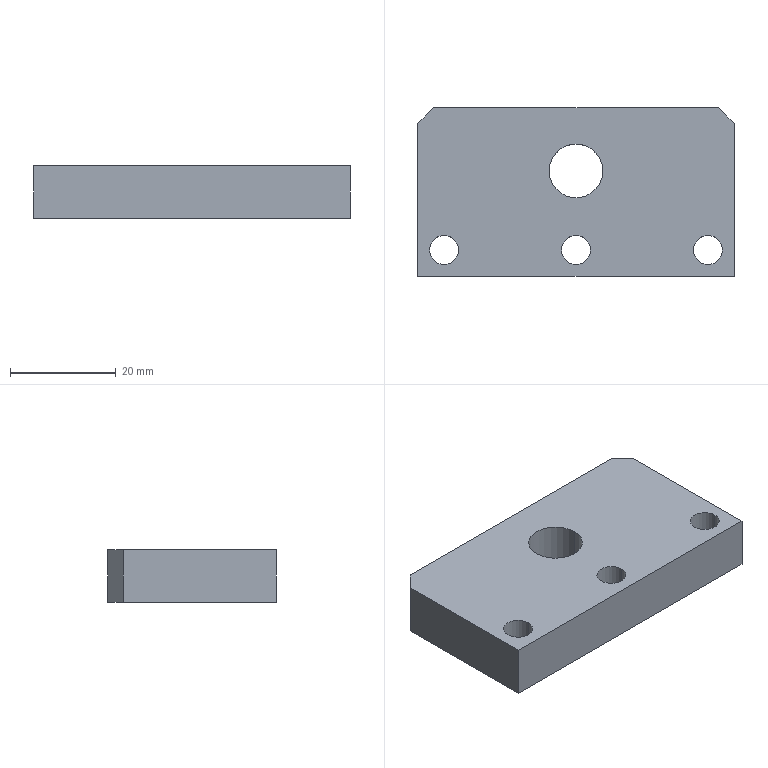Part | STEP file | MT-COMBO-119-S030 | 1 solid | 16 faces | box 60 x 32 x 10 mm | volume 17580 mm3 | cylinder 8 | plane 8 | commonest cylinder face diameters 5.5 x6 10.2 x2
STEP:
#1=CARTESIAN_POINT('',(-22.25,-11.,5.));
#2=VERTEX_POINT('',#1);
#3=CARTESIAN_POINT('',(-27.75,-11.,5.));
#4=VERTEX_POINT('',#3);
#5=CARTESIAN_POINT('',(-25.,-11.,5.));
#6=DIRECTION('',(0.,0.,1.));
#7=DIRECTION('',(1.,0.,0.));
#8=AXIS2_PLACEMENT_3D('',#5,#6,#7);
#9=CIRCLE('',#8,2.75);
#10=EDGE_CURVE('',#2,#4,#9,.T.);
#11=ORIENTED_EDGE('',*,*,#10,.T.);
#12=CARTESIAN_POINT('',(-27.75,-11.,-5.));
#13=VERTEX_POINT('',#12);
#14=CARTESIAN_POINT('',(-27.75,-11.,-5.));
#15=DIRECTION('',(0.,0.,-1.));
#16=VECTOR('',#15,1000.);
#17=LINE('',#14,#16);
#18=EDGE_CURVE('',#4,#13,#17,.T.);
#19=ORIENTED_EDGE('',*,*,#18,.T.);
#20=CARTESIAN_POINT('',(-22.25,-11.,-5.));
#21=VERTEX_POINT('',#20);
#22=CARTESIAN_POINT('',(-25.,-11.,-5.));
#23=DIRECTION('',(0.,0.,1.));
#24=DIRECTION('',(1.,0.,0.));
#25=AXIS2_PLACEMENT_3D('',#22,#23,#24);
#26=CIRCLE('',#25,2.75);
#27=EDGE_CURVE('',#21,#13,#26,.T.);
#28=ORIENTED_EDGE('',*,*,#27,.F.);
#29=CARTESIAN_POINT('',(-22.25,-11.,-5.));
#30=DIRECTION('',(0.,0.,-1.));
#31=VECTOR('',#30,1000.);
#32=LINE('',#29,#31);
#33=EDGE_CURVE('',#2,#21,#32,.T.);
#34=ORIENTED_EDGE('',*,*,#33,.F.);
#35=EDGE_LOOP('',(#11,#19,#28,#34));
#36=FACE_OUTER_BOUND('',#35,.T.);
#37=CARTESIAN_POINT('',(-25.,-11.,-5.));
#38=DIRECTION('',(0.,0.,-1.));
#39=DIRECTION('',(1.,0.,0.));
#40=AXIS2_PLACEMENT_3D('',#37,#38,#39);
#41=CYLINDRICAL_SURFACE('',#40,2.75);
#42=ADVANCED_FACE('',(#36),#41,.F.);
#43=CARTESIAN_POINT('',(27.75,-11.,5.));
#44=VERTEX_POINT('',#43);
#45=CARTESIAN_POINT('',(22.25,-11.,5.));
#46=VERTEX_POINT('',#45);
#47=CARTESIAN_POINT('',(25.,-11.,5.));
#48=DIRECTION('',(0.,0.,1.));
#49=DIRECTION('',(1.,0.,0.));
#50=AXIS2_PLACEMENT_3D('',#47,#48,#49);
#51=CIRCLE('',#50,2.75);
#52=EDGE_CURVE('',#44,#46,#51,.T.);
#53=ORIENTED_EDGE('',*,*,#52,.T.);
#54=CARTESIAN_POINT('',(22.25,-11.,-5.));
#55=VERTEX_POINT('',#54);
#56=CARTESIAN_POINT('',(22.25,-11.,-5.));
#57=DIRECTION('',(0.,0.,-1.));
#58=VECTOR('',#57,1000.);
#59=LINE('',#56,#58);
#60=EDGE_CURVE('',#46,#55,#59,.T.);
#61=ORIENTED_EDGE('',*,*,#60,.T.);
#62=CARTESIAN_POINT('',(27.75,-11.,-5.));
#63=VERTEX_POINT('',#62);
#64=CARTESIAN_POINT('',(25.,-11.,-5.));
#65=DIRECTION('',(0.,0.,1.));
#66=DIRECTION('',(1.,0.,0.));
#67=AXIS2_PLACEMENT_3D('',#64,#65,#66);
#68=CIRCLE('',#67,2.75);
#69=EDGE_CURVE('',#63,#55,#68,.T.);
#70=ORIENTED_EDGE('',*,*,#69,.F.);
#71=CARTESIAN_POINT('',(27.75,-11.,-5.));
#72=DIRECTION('',(0.,0.,-1.));
#73=VECTOR('',#72,1000.);
#74=LINE('',#71,#73);
#75=EDGE_CURVE('',#44,#63,#74,.T.);
#76=ORIENTED_EDGE('',*,*,#75,.F.);
#77=EDGE_LOOP('',(#53,#61,#70,#76));
#78=FACE_OUTER_BOUND('',#77,.T.);
#79=CARTESIAN_POINT('',(25.,-11.,-5.));
#80=DIRECTION('',(0.,0.,-1.));
#81=DIRECTION('',(1.,0.,0.));
#82=AXIS2_PLACEMENT_3D('',#79,#80,#81);
#83=CYLINDRICAL_SURFACE('',#82,2.75);
#84=ADVANCED_FACE('',(#78),#83,.F.);
#85=CARTESIAN_POINT('',(2.75,-11.,5.));
#86=VERTEX_POINT('',#85);
#87=CARTESIAN_POINT('',(-2.75,-11.,5.));
#88=VERTEX_POINT('',#87);
#89=CARTESIAN_POINT('',(0.,-11.,5.));
#90=DIRECTION('',(0.,0.,1.));
#91=DIRECTION('',(1.,0.,0.));
#92=AXIS2_PLACEMENT_3D('',#89,#90,#91);
#93=CIRCLE('',#92,2.75);
#94=EDGE_CURVE('',#86,#88,#93,.T.);
#95=ORIENTED_EDGE('',*,*,#94,.T.);
#96=CARTESIAN_POINT('',(-2.75,-11.,-5.));
#97=VERTEX_POINT('',#96);
#98=CARTESIAN_POINT('',(-2.75,-11.,-5.));
#99=DIRECTION('',(0.,0.,-1.));
#100=VECTOR('',#99,1000.);
#101=LINE('',#98,#100);
#102=EDGE_CURVE('',#88,#97,#101,.T.);
#103=ORIENTED_EDGE('',*,*,#102,.T.);
#104=CARTESIAN_POINT('',(2.75,-11.,-5.));
#105=VERTEX_POINT('',#104);
#106=CARTESIAN_POINT('',(0.,-11.,-5.));
#107=DIRECTION('',(0.,0.,1.));
#108=DIRECTION('',(1.,0.,0.));
#109=AXIS2_PLACEMENT_3D('',#106,#107,#108);
#110=CIRCLE('',#109,2.75);
#111=EDGE_CURVE('',#105,#97,#110,.T.);
#112=ORIENTED_EDGE('',*,*,#111,.F.);
#113=CARTESIAN_POINT('',(2.75,-11.,-5.));
#114=DIRECTION('',(0.,0.,-1.));
#115=VECTOR('',#114,1000.);
#116=LINE('',#113,#115);
#117=EDGE_CURVE('',#86,#105,#116,.T.);
#118=ORIENTED_EDGE('',*,*,#117,.F.);
#119=EDGE_LOOP('',(#95,#103,#112,#118));
#120=FACE_OUTER_BOUND('',#119,.T.);
#121=CARTESIAN_POINT('',(0.,-11.,-5.));
#122=DIRECTION('',(0.,0.,-1.));
#123=DIRECTION('',(1.,0.,0.));
#124=AXIS2_PLACEMENT_3D('',#121,#122,#123);
#125=CYLINDRICAL_SURFACE('',#124,2.75);
#126=ADVANCED_FACE('',(#120),#125,.F.);
#127=CARTESIAN_POINT('',(5.1,4.,5.));
#128=VERTEX_POINT('',#127);
#129=CARTESIAN_POINT('',(-5.1,4.,5.));
#130=VERTEX_POINT('',#129);
#131=CARTESIAN_POINT('',(0.,4.,5.));
#132=DIRECTION('',(0.,0.,1.));
#133=DIRECTION('',(1.,0.,0.));
#134=AXIS2_PLACEMENT_3D('',#131,#132,#133);
#135=CIRCLE('',#134,5.1);
#136=EDGE_CURVE('',#128,#130,#135,.T.);
#137=ORIENTED_EDGE('',*,*,#136,.T.);
#138=CARTESIAN_POINT('',(-5.1,4.,-5.));
#139=VERTEX_POINT('',#138);
#140=CARTESIAN_POINT('',(-5.1,4.,-5.));
#141=DIRECTION('',(0.,0.,-1.));
#142=VECTOR('',#141,1000.);
#143=LINE('',#140,#142);
#144=EDGE_CURVE('',#130,#139,#143,.T.);
#145=ORIENTED_EDGE('',*,*,#144,.T.);
#146=CARTESIAN_POINT('',(5.1,4.,-5.));
#147=VERTEX_POINT('',#146);
#148=CARTESIAN_POINT('',(0.,4.,-5.));
#149=DIRECTION('',(0.,0.,1.));
#150=DIRECTION('',(1.,0.,0.));
#151=AXIS2_PLACEMENT_3D('',#148,#149,#150);
#152=CIRCLE('',#151,5.1);
#153=EDGE_CURVE('',#147,#139,#152,.T.);
#154=ORIENTED_EDGE('',*,*,#153,.F.);
#155=CARTESIAN_POINT('',(5.1,4.,-5.));
#156=DIRECTION('',(0.,0.,-1.));
#157=VECTOR('',#156,1000.);
#158=LINE('',#155,#157);
#159=EDGE_CURVE('',#128,#147,#158,.T.);
#160=ORIENTED_EDGE('',*,*,#159,.F.);
#161=EDGE_LOOP('',(#137,#145,#154,#160));
#162=FACE_OUTER_BOUND('',#161,.T.);
#163=CARTESIAN_POINT('',(0.,4.,-5.));
#164=DIRECTION('',(0.,0.,-1.));
#165=DIRECTION('',(1.,0.,0.));
#166=AXIS2_PLACEMENT_3D('',#163,#164,#165);
#167=CYLINDRICAL_SURFACE('',#166,5.1);
#168=ADVANCED_FACE('',(#162),#167,.F.);
#169=CARTESIAN_POINT('',(30.,-16.,5.));
#170=VERTEX_POINT('',#169);
#171=CARTESIAN_POINT('',(30.,13.,5.));
#172=VERTEX_POINT('',#171);
#173=CARTESIAN_POINT('',(30.,16.,5.));
#174=DIRECTION('',(0.,1.,0.));
#175=VECTOR('',#174,1000.);
#176=LINE('',#173,#175);
#177=EDGE_CURVE('',#170,#172,#176,.T.);
#178=ORIENTED_EDGE('',*,*,#177,.F.);
#179=CARTESIAN_POINT('',(30.,-16.,-5.));
#180=VERTEX_POINT('',#179);
#181=CARTESIAN_POINT('',(30.,-16.,-5.));
#182=DIRECTION('',(0.,0.,1.));
#183=VECTOR('',#182,1000.);
#184=LINE('',#181,#183);
#185=EDGE_CURVE('',#180,#170,#184,.T.);
#186=ORIENTED_EDGE('',*,*,#185,.F.);
#187=CARTESIAN_POINT('',(30.,13.,-5.));
#188=VERTEX_POINT('',#187);
#189=CARTESIAN_POINT('',(30.,16.,-5.));
#190=DIRECTION('',(0.,1.,0.));
#191=VECTOR('',#190,1000.);
#192=LINE('',#189,#191);
#193=EDGE_CURVE('',#180,#188,#192,.T.);
#194=ORIENTED_EDGE('',*,*,#193,.T.);
#195=CARTESIAN_POINT('',(30.,13.,-5.));
#196=DIRECTION('',(0.,0.,-1.));
#197=VECTOR('',#196,1000.);
#198=LINE('',#195,#197);
#199=EDGE_CURVE('',#172,#188,#198,.T.);
#200=ORIENTED_EDGE('',*,*,#199,.F.);
#201=EDGE_LOOP('',(#178,#186,#194,#200));
#202=FACE_OUTER_BOUND('',#201,.T.);
#203=CARTESIAN_POINT('',(30.,16.,-5.));
#204=DIRECTION('',(-1.,0.,0.));
#205=DIRECTION('',(0.,-1.,0.));
#206=AXIS2_PLACEMENT_3D('',#203,#204,#205);
#207=PLANE('',#206);
#208=ADVANCED_FACE('',(#202),#207,.F.);
#209=CARTESIAN_POINT('',(27.,16.,-5.));
#210=VERTEX_POINT('',#209);
#211=CARTESIAN_POINT('',(-27.,16.,-5.));
#212=VERTEX_POINT('',#211);
#213=CARTESIAN_POINT('',(-30.,16.,-5.));
#214=DIRECTION('',(-1.,0.,0.));
#215=VECTOR('',#214,1000.);
#216=LINE('',#213,#215);
#217=EDGE_CURVE('',#210,#212,#216,.T.);
#218=ORIENTED_EDGE('',*,*,#217,.T.);
#219=CARTESIAN_POINT('',(-27.,16.,5.));
#220=VERTEX_POINT('',#219);
#221=CARTESIAN_POINT('',(-27.,16.,-5.));
#222=DIRECTION('',(0.,0.,-1.));
#223=VECTOR('',#222,1000.);
#224=LINE('',#221,#223);
#225=EDGE_CURVE('',#220,#212,#224,.T.);
#226=ORIENTED_EDGE('',*,*,#225,.F.);
#227=CARTESIAN_POINT('',(27.,16.,5.));
#228=VERTEX_POINT('',#227);
#229=CARTESIAN_POINT('',(-30.,16.,5.));
#230=DIRECTION('',(-1.,0.,0.));
#231=VECTOR('',#230,1000.);
#232=LINE('',#229,#231);
#233=EDGE_CURVE('',#228,#220,#232,.T.);
#234=ORIENTED_EDGE('',*,*,#233,.F.);
#235=CARTESIAN_POINT('',(27.,16.,-5.));
#236=DIRECTION('',(0.,0.,1.));
#237=VECTOR('',#236,1000.);
#238=LINE('',#235,#237);
#239=EDGE_CURVE('',#210,#228,#238,.T.);
#240=ORIENTED_EDGE('',*,*,#239,.F.);
#241=EDGE_LOOP('',(#218,#226,#234,#240));
#242=FACE_OUTER_BOUND('',#241,.T.);
#243=CARTESIAN_POINT('',(-30.,16.,-5.));
#244=DIRECTION('',(0.,-1.,0.));
#245=DIRECTION('',(0.,0.,1.));
#246=AXIS2_PLACEMENT_3D('',#243,#244,#245);
#247=PLANE('',#246);
#248=ADVANCED_FACE('',(#242),#247,.F.);
#249=CARTESIAN_POINT('',(-30.,13.,-5.));
#250=VERTEX_POINT('',#249);
#251=CARTESIAN_POINT('',(-30.,-16.,-5.));
#252=VERTEX_POINT('',#251);
#253=CARTESIAN_POINT('',(-30.,16.,-5.));
#254=DIRECTION('',(0.,-1.,0.));
#255=VECTOR('',#254,1000.);
#256=LINE('',#253,#255);
#257=EDGE_CURVE('',#250,#252,#256,.T.);
#258=ORIENTED_EDGE('',*,*,#257,.T.);
#259=CARTESIAN_POINT('',(-30.,-16.,5.));
#260=VERTEX_POINT('',#259);
#261=CARTESIAN_POINT('',(-30.,-16.,-5.));
#262=DIRECTION('',(0.,0.,1.));
#263=VECTOR('',#262,1000.);
#264=LINE('',#261,#263);
#265=EDGE_CURVE('',#252,#260,#264,.T.);
#266=ORIENTED_EDGE('',*,*,#265,.T.);
#267=CARTESIAN_POINT('',(-30.,13.,5.));
#268=VERTEX_POINT('',#267);
#269=CARTESIAN_POINT('',(-30.,16.,5.));
#270=DIRECTION('',(0.,-1.,0.));
#271=VECTOR('',#270,1000.);
#272=LINE('',#269,#271);
#273=EDGE_CURVE('',#268,#260,#272,.T.);
#274=ORIENTED_EDGE('',*,*,#273,.F.);
#275=CARTESIAN_POINT('',(-30.,13.,-5.));
#276=DIRECTION('',(0.,0.,1.));
#277=VECTOR('',#276,1000.);
#278=LINE('',#275,#277);
#279=EDGE_CURVE('',#250,#268,#278,.T.);
#280=ORIENTED_EDGE('',*,*,#279,.F.);
#281=EDGE_LOOP('',(#258,#266,#274,#280));
#282=FACE_OUTER_BOUND('',#281,.T.);
#283=CARTESIAN_POINT('',(-30.,16.,-5.));
#284=DIRECTION('',(1.,0.,0.));
#285=DIRECTION('',(0.,1.,0.));
#286=AXIS2_PLACEMENT_3D('',#283,#284,#285);
#287=PLANE('',#286);
#288=ADVANCED_FACE('',(#282),#287,.F.);
#289=CARTESIAN_POINT('',(-30.,-16.,5.));
#290=DIRECTION('',(1.,0.,0.));
#291=VECTOR('',#290,1000.);
#292=LINE('',#289,#291);
#293=EDGE_CURVE('',#260,#170,#292,.T.);
#294=ORIENTED_EDGE('',*,*,#293,.F.);
#295=ORIENTED_EDGE('',*,*,#265,.F.);
#296=CARTESIAN_POINT('',(-30.,-16.,-5.));
#297=DIRECTION('',(1.,0.,0.));
#298=VECTOR('',#297,1000.);
#299=LINE('',#296,#298);
#300=EDGE_CURVE('',#252,#180,#299,.T.);
#301=ORIENTED_EDGE('',*,*,#300,.T.);
#302=ORIENTED_EDGE('',*,*,#185,.T.);
#303=EDGE_LOOP('',(#294,#295,#301,#302));
#304=FACE_OUTER_BOUND('',#303,.T.);
#305=CARTESIAN_POINT('',(-30.,-16.,-5.));
#306=DIRECTION('',(0.,1.,0.));
#307=DIRECTION('',(0.,0.,-1.));
#308=AXIS2_PLACEMENT_3D('',#305,#306,#307);
#309=PLANE('',#308);
#310=ADVANCED_FACE('',(#304),#309,.F.);
#311=ORIENTED_EDGE('',*,*,#27,.T.);
#312=CARTESIAN_POINT('',(-25.,-11.,-5.));
#313=DIRECTION('',(0.,0.,1.));
#314=DIRECTION('',(1.,0.,0.));
#315=AXIS2_PLACEMENT_3D('',#312,#313,#314);
#316=CIRCLE('',#315,2.75);
#317=EDGE_CURVE('',#13,#21,#316,.T.);
#318=ORIENTED_EDGE('',*,*,#317,.T.);
#319=EDGE_LOOP('',(#311,#318));
#320=FACE_BOUND('',#319,.T.);
#321=ORIENTED_EDGE('',*,*,#69,.T.);
#322=CARTESIAN_POINT('',(25.,-11.,-5.));
#323=DIRECTION('',(0.,0.,1.));
#324=DIRECTION('',(1.,0.,0.));
#325=AXIS2_PLACEMENT_3D('',#322,#323,#324);
#326=CIRCLE('',#325,2.75);
#327=EDGE_CURVE('',#55,#63,#326,.T.);
#328=ORIENTED_EDGE('',*,*,#327,.T.);
#329=EDGE_LOOP('',(#321,#328));
#330=FACE_BOUND('',#329,.T.);
#331=ORIENTED_EDGE('',*,*,#111,.T.);
#332=CARTESIAN_POINT('',(0.,-11.,-5.));
#333=DIRECTION('',(0.,0.,1.));
#334=DIRECTION('',(1.,0.,0.));
#335=AXIS2_PLACEMENT_3D('',#332,#333,#334);
#336=CIRCLE('',#335,2.75);
#337=EDGE_CURVE('',#97,#105,#336,.T.);
#338=ORIENTED_EDGE('',*,*,#337,.T.);
#339=EDGE_LOOP('',(#331,#338));
#340=FACE_BOUND('',#339,.T.);
#341=ORIENTED_EDGE('',*,*,#153,.T.);
#342=CARTESIAN_POINT('',(0.,4.,-5.));
#343=DIRECTION('',(0.,0.,1.));
#344=DIRECTION('',(1.,0.,0.));
#345=AXIS2_PLACEMENT_3D('',#342,#343,#344);
#346=CIRCLE('',#345,5.1);
#347=EDGE_CURVE('',#139,#147,#346,.T.);
#348=ORIENTED_EDGE('',*,*,#347,.T.);
#349=EDGE_LOOP('',(#341,#348));
#350=FACE_BOUND('',#349,.T.);
#351=ORIENTED_EDGE('',*,*,#193,.F.);
#352=ORIENTED_EDGE('',*,*,#300,.F.);
#353=ORIENTED_EDGE('',*,*,#257,.F.);
#354=CARTESIAN_POINT('',(-21.5,21.5,-5.));
#355=DIRECTION('',(-0.7071,-0.7071,0.));
#356=VECTOR('',#355,1000.);
#357=LINE('',#354,#356);
#358=EDGE_CURVE('',#212,#250,#357,.T.);
#359=ORIENTED_EDGE('',*,*,#358,.F.);
#360=ORIENTED_EDGE('',*,*,#217,.F.);
#361=CARTESIAN_POINT('',(21.5,21.5,-5.));
#362=DIRECTION('',(-0.7071,0.7071,0.));
#363=VECTOR('',#362,1000.);
#364=LINE('',#361,#363);
#365=EDGE_CURVE('',#188,#210,#364,.T.);
#366=ORIENTED_EDGE('',*,*,#365,.F.);
#367=EDGE_LOOP('',(#351,#352,#353,#359,#360,#366));
#368=FACE_OUTER_BOUND('',#367,.T.);
#369=CARTESIAN_POINT('',(0.,0.,-5.));
#370=DIRECTION('',(0.,0.,-1.));
#371=DIRECTION('',(1.,0.,0.));
#372=AXIS2_PLACEMENT_3D('',#369,#370,#371);
#373=PLANE('',#372);
#374=ADVANCED_FACE('',(#320,#330,#340,#350,#368),#373,.T.);
#375=ORIENTED_EDGE('',*,*,#10,.F.);
#376=CARTESIAN_POINT('',(-25.,-11.,5.));
#377=DIRECTION('',(0.,0.,1.));
#378=DIRECTION('',(1.,0.,0.));
#379=AXIS2_PLACEMENT_3D('',#376,#377,#378);
#380=CIRCLE('',#379,2.75);
#381=EDGE_CURVE('',#4,#2,#380,.T.);
#382=ORIENTED_EDGE('',*,*,#381,.F.);
#383=EDGE_LOOP('',(#375,#382));
#384=FACE_BOUND('',#383,.T.);
#385=ORIENTED_EDGE('',*,*,#52,.F.);
#386=CARTESIAN_POINT('',(25.,-11.,5.));
#387=DIRECTION('',(0.,0.,1.));
#388=DIRECTION('',(1.,0.,0.));
#389=AXIS2_PLACEMENT_3D('',#386,#387,#388);
#390=CIRCLE('',#389,2.75);
#391=EDGE_CURVE('',#46,#44,#390,.T.);
#392=ORIENTED_EDGE('',*,*,#391,.F.);
#393=EDGE_LOOP('',(#385,#392));
#394=FACE_BOUND('',#393,.T.);
#395=ORIENTED_EDGE('',*,*,#94,.F.);
#396=CARTESIAN_POINT('',(0.,-11.,5.));
#397=DIRECTION('',(0.,0.,1.));
#398=DIRECTION('',(1.,0.,0.));
#399=AXIS2_PLACEMENT_3D('',#396,#397,#398);
#400=CIRCLE('',#399,2.75);
#401=EDGE_CURVE('',#88,#86,#400,.T.);
#402=ORIENTED_EDGE('',*,*,#401,.F.);
#403=EDGE_LOOP('',(#395,#402));
#404=FACE_BOUND('',#403,.T.);
#405=ORIENTED_EDGE('',*,*,#136,.F.);
#406=CARTESIAN_POINT('',(0.,4.,5.));
#407=DIRECTION('',(0.,0.,1.));
#408=DIRECTION('',(1.,0.,0.));
#409=AXIS2_PLACEMENT_3D('',#406,#407,#408);
#410=CIRCLE('',#409,5.1);
#411=EDGE_CURVE('',#130,#128,#410,.T.);
#412=ORIENTED_EDGE('',*,*,#411,.F.);
#413=EDGE_LOOP('',(#405,#412));
#414=FACE_BOUND('',#413,.T.);
#415=ORIENTED_EDGE('',*,*,#233,.T.);
#416=CARTESIAN_POINT('',(-30.,13.,5.));
#417=DIRECTION('',(0.7071,0.7071,0.));
#418=VECTOR('',#417,1000.);
#419=LINE('',#416,#418);
#420=EDGE_CURVE('',#268,#220,#419,.T.);
#421=ORIENTED_EDGE('',*,*,#420,.F.);
#422=ORIENTED_EDGE('',*,*,#273,.T.);
#423=ORIENTED_EDGE('',*,*,#293,.T.);
#424=ORIENTED_EDGE('',*,*,#177,.T.);
#425=CARTESIAN_POINT('',(27.,16.,5.));
#426=DIRECTION('',(0.7071,-0.7071,0.));
#427=VECTOR('',#426,1000.);
#428=LINE('',#425,#427);
#429=EDGE_CURVE('',#228,#172,#428,.T.);
#430=ORIENTED_EDGE('',*,*,#429,.F.);
#431=EDGE_LOOP('',(#415,#421,#422,#423,#424,#430));
#432=FACE_OUTER_BOUND('',#431,.T.);
#433=CARTESIAN_POINT('',(0.,0.,5.));
#434=DIRECTION('',(0.,0.,-1.));
#435=DIRECTION('',(1.,0.,0.));
#436=AXIS2_PLACEMENT_3D('',#433,#434,#435);
#437=PLANE('',#436);
#438=ADVANCED_FACE('',(#384,#394,#404,#414,#432),#437,.F.);
#439=ORIENTED_EDGE('',*,*,#144,.F.);
#440=ORIENTED_EDGE('',*,*,#411,.T.);
#441=ORIENTED_EDGE('',*,*,#159,.T.);
#442=ORIENTED_EDGE('',*,*,#347,.F.);
#443=EDGE_LOOP('',(#439,#440,#441,#442));
#444=FACE_OUTER_BOUND('',#443,.T.);
#445=CARTESIAN_POINT('',(0.,4.,-5.));
#446=DIRECTION('',(0.,0.,-1.));
#447=DIRECTION('',(1.,0.,0.));
#448=AXIS2_PLACEMENT_3D('',#445,#446,#447);
#449=CYLINDRICAL_SURFACE('',#448,5.1);
#450=ADVANCED_FACE('',(#444),#449,.F.);
#451=ORIENTED_EDGE('',*,*,#102,.F.);
#452=ORIENTED_EDGE('',*,*,#401,.T.);
#453=ORIENTED_EDGE('',*,*,#117,.T.);
#454=ORIENTED_EDGE('',*,*,#337,.F.);
#455=EDGE_LOOP('',(#451,#452,#453,#454));
#456=FACE_OUTER_BOUND('',#455,.T.);
#457=CARTESIAN_POINT('',(0.,-11.,-5.));
#458=DIRECTION('',(0.,0.,-1.));
#459=DIRECTION('',(1.,0.,0.));
#460=AXIS2_PLACEMENT_3D('',#457,#458,#459);
#461=CYLINDRICAL_SURFACE('',#460,2.75);
#462=ADVANCED_FACE('',(#456),#461,.F.);
#463=ORIENTED_EDGE('',*,*,#60,.F.);
#464=ORIENTED_EDGE('',*,*,#391,.T.);
#465=ORIENTED_EDGE('',*,*,#75,.T.);
#466=ORIENTED_EDGE('',*,*,#327,.F.);
#467=EDGE_LOOP('',(#463,#464,#465,#466));
#468=FACE_OUTER_BOUND('',#467,.T.);
#469=CARTESIAN_POINT('',(25.,-11.,-5.));
#470=DIRECTION('',(0.,0.,-1.));
#471=DIRECTION('',(1.,0.,0.));
#472=AXIS2_PLACEMENT_3D('',#469,#470,#471);
#473=CYLINDRICAL_SURFACE('',#472,2.75);
#474=ADVANCED_FACE('',(#468),#473,.F.);
#475=ORIENTED_EDGE('',*,*,#18,.F.);
#476=ORIENTED_EDGE('',*,*,#381,.T.);
#477=ORIENTED_EDGE('',*,*,#33,.T.);
#478=ORIENTED_EDGE('',*,*,#317,.F.);
#479=EDGE_LOOP('',(#475,#476,#477,#478));
#480=FACE_OUTER_BOUND('',#479,.T.);
#481=CARTESIAN_POINT('',(-25.,-11.,-5.));
#482=DIRECTION('',(0.,0.,-1.));
#483=DIRECTION('',(1.,0.,0.));
#484=AXIS2_PLACEMENT_3D('',#481,#482,#483);
#485=CYLINDRICAL_SURFACE('',#484,2.75);
#486=ADVANCED_FACE('',(#480),#485,.F.);
#487=ORIENTED_EDGE('',*,*,#365,.T.);
#488=ORIENTED_EDGE('',*,*,#239,.T.);
#489=ORIENTED_EDGE('',*,*,#429,.T.);
#490=ORIENTED_EDGE('',*,*,#199,.T.);
#491=EDGE_LOOP('',(#487,#488,#489,#490));
#492=FACE_OUTER_BOUND('',#491,.T.);
#493=CARTESIAN_POINT('',(27.,16.,-5.));
#494=DIRECTION('',(-0.7071,-0.7071,0.));
#495=DIRECTION('',(0.,0.,1.));
#496=AXIS2_PLACEMENT_3D('',#493,#494,#495);
#497=PLANE('',#496);
#498=ADVANCED_FACE('',(#492),#497,.F.);
#499=ORIENTED_EDGE('',*,*,#358,.T.);
#500=ORIENTED_EDGE('',*,*,#279,.T.);
#501=ORIENTED_EDGE('',*,*,#420,.T.);
#502=ORIENTED_EDGE('',*,*,#225,.T.);
#503=EDGE_LOOP('',(#499,#500,#501,#502));
#504=FACE_OUTER_BOUND('',#503,.T.);
#505=CARTESIAN_POINT('',(-30.,13.,-5.));
#506=DIRECTION('',(0.7071,-0.7071,0.));
#507=DIRECTION('',(0.,0.,1.));
#508=AXIS2_PLACEMENT_3D('',#505,#506,#507);
#509=PLANE('',#508);
#510=ADVANCED_FACE('',(#504),#509,.F.);
#511=CLOSED_SHELL('',(#42,#84,#126,#168,#208,#248,#288,#310,#374,#438,#450,#462,#474,#486,#498,#510));
#512=MANIFOLD_SOLID_BREP('',#511);
#513=CARTESIAN_POINT('',(0.,0.,0.));
#514=DIRECTION('',(0.,0.,1.));
#515=DIRECTION('',(1.,0.,0.));
#516=AXIS2_PLACEMENT_3D('',#513,#514,#515);
#517=(LENGTH_UNIT()NAMED_UNIT(*)SI_UNIT(.MILLI.,.METRE.));
#518=UNCERTAINTY_MEASURE_WITH_UNIT(LENGTH_MEASURE(0.00001),#517,'','');
#519=(NAMED_UNIT(*)PLANE_ANGLE_UNIT()SI_UNIT($,.RADIAN.));
#520=(NAMED_UNIT(*)SI_UNIT($,.STERADIAN.)SOLID_ANGLE_UNIT());
#521=(GEOMETRIC_REPRESENTATION_CONTEXT(3)GLOBAL_UNCERTAINTY_ASSIGNED_CONTEXT((#518))GLOBAL_UNIT_ASSIGNED_CONTEXT((#517,#519,#520))REPRESENTATION_CONTEXT('',''));
#522=ADVANCED_BREP_SHAPE_REPRESENTATION('',(#512,#516),#521);